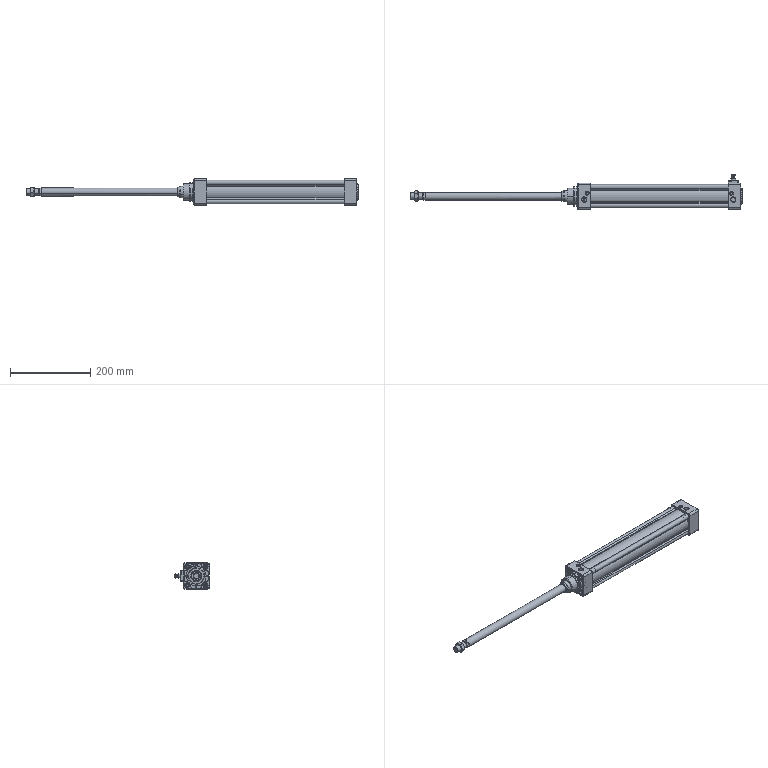Part | SolidWorks | 15 solids | 907 faces | box 828.5 x 86 x 65 mm | volume 699915 mm3 | plane 346 | cylinder 259 | cone 240 | spline 62 | commonest cylinder face diameters 12 x32 8 x20 2 x16 6.647 x16 8.7 x16 12.7 x16